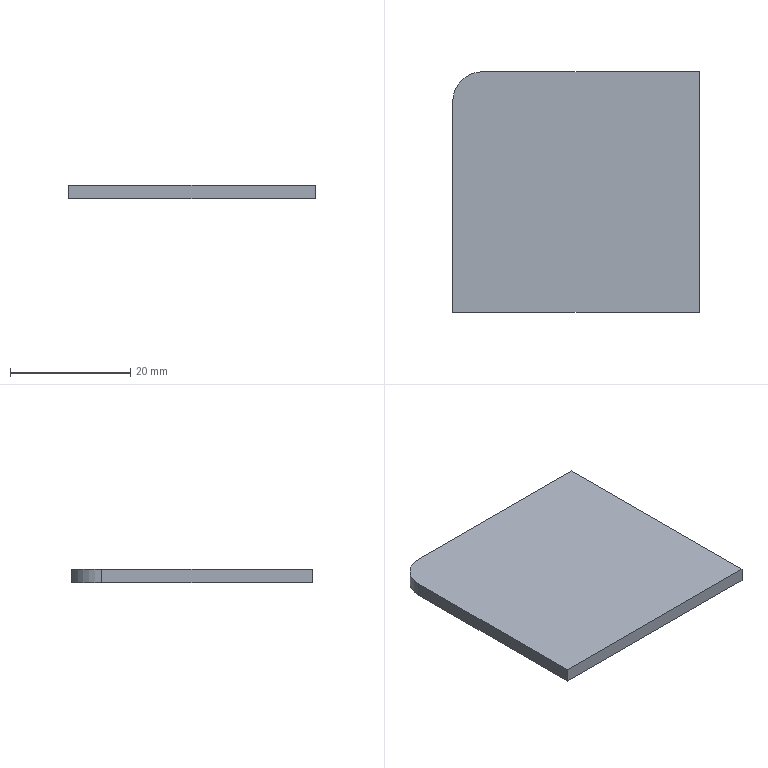Part | SolidWorks | features FlatPattern 1, SMBaseFlange 1, SheetMetal 1 | 1 solid | 7 faces | box 41 x 40 x 2.3 mm | volume 3760 mm3 | plane 6 | cylinder 1 | commonest cylinder face diameters 10 x1
STEP:
#1=CARTESIAN_POINT('',(41.,-40.,0.));
#2=VERTEX_POINT('',#1);
#3=CARTESIAN_POINT('',(41.,0.,0.));
#4=VERTEX_POINT('',#3);
#5=CARTESIAN_POINT('',(41.,0.,0.));
#6=DIRECTION('',(0.,1.,0.));
#7=VECTOR('',#6,1000.);
#8=LINE('',#5,#7);
#9=EDGE_CURVE('',#2,#4,#8,.T.);
#10=ORIENTED_EDGE('',*,*,#9,.F.);
#11=CARTESIAN_POINT('',(41.,-40.,-2.3));
#12=VERTEX_POINT('',#11);
#13=CARTESIAN_POINT('',(41.,-40.,-2.3));
#14=DIRECTION('',(0.,0.,1.));
#15=VECTOR('',#14,1000.);
#16=LINE('',#13,#15);
#17=EDGE_CURVE('',#12,#2,#16,.T.);
#18=ORIENTED_EDGE('',*,*,#17,.F.);
#19=CARTESIAN_POINT('',(41.,0.,-2.3));
#20=VERTEX_POINT('',#19);
#21=CARTESIAN_POINT('',(41.,0.,-2.3));
#22=DIRECTION('',(0.,1.,0.));
#23=VECTOR('',#22,1000.);
#24=LINE('',#21,#23);
#25=EDGE_CURVE('',#12,#20,#24,.T.);
#26=ORIENTED_EDGE('',*,*,#25,.T.);
#27=CARTESIAN_POINT('',(41.,0.,-2.3));
#28=DIRECTION('',(0.,0.,1.));
#29=VECTOR('',#28,1000.);
#30=LINE('',#27,#29);
#31=EDGE_CURVE('',#20,#4,#30,.T.);
#32=ORIENTED_EDGE('',*,*,#31,.T.);
#33=EDGE_LOOP('',(#10,#18,#26,#32));
#34=FACE_OUTER_BOUND('',#33,.T.);
#35=CARTESIAN_POINT('',(41.,0.,-2.3));
#36=DIRECTION('',(1.,0.,0.));
#37=DIRECTION('',(0.,1.,0.));
#38=AXIS2_PLACEMENT_3D('',#35,#36,#37);
#39=PLANE('',#38);
#40=ADVANCED_FACE('',(#34),#39,.T.);
#41=CARTESIAN_POINT('',(0.,-40.,0.));
#42=VERTEX_POINT('',#41);
#43=CARTESIAN_POINT('',(0.,-40.,0.));
#44=DIRECTION('',(1.,0.,0.));
#45=VECTOR('',#44,1000.);
#46=LINE('',#43,#45);
#47=EDGE_CURVE('',#42,#2,#46,.T.);
#48=ORIENTED_EDGE('',*,*,#47,.F.);
#49=CARTESIAN_POINT('',(0.,-40.,-2.3));
#50=VERTEX_POINT('',#49);
#51=CARTESIAN_POINT('',(0.,-40.,-2.3));
#52=DIRECTION('',(0.,0.,1.));
#53=VECTOR('',#52,1000.);
#54=LINE('',#51,#53);
#55=EDGE_CURVE('',#50,#42,#54,.T.);
#56=ORIENTED_EDGE('',*,*,#55,.F.);
#57=CARTESIAN_POINT('',(0.,-40.,-2.3));
#58=DIRECTION('',(1.,0.,0.));
#59=VECTOR('',#58,1000.);
#60=LINE('',#57,#59);
#61=EDGE_CURVE('',#50,#12,#60,.T.);
#62=ORIENTED_EDGE('',*,*,#61,.T.);
#63=ORIENTED_EDGE('',*,*,#17,.T.);
#64=EDGE_LOOP('',(#48,#56,#62,#63));
#65=FACE_OUTER_BOUND('',#64,.T.);
#66=CARTESIAN_POINT('',(0.,-40.,-2.3));
#67=DIRECTION('',(0.,-1.,0.));
#68=DIRECTION('',(0.,0.,-1.));
#69=AXIS2_PLACEMENT_3D('',#66,#67,#68);
#70=PLANE('',#69);
#71=ADVANCED_FACE('',(#65),#70,.T.);
#72=CARTESIAN_POINT('',(0.,-5.,0.));
#73=VERTEX_POINT('',#72);
#74=CARTESIAN_POINT('',(0.,-5.,0.));
#75=DIRECTION('',(0.,-1.,0.));
#76=VECTOR('',#75,1000.);
#77=LINE('',#74,#76);
#78=EDGE_CURVE('',#73,#42,#77,.T.);
#79=ORIENTED_EDGE('',*,*,#78,.F.);
#80=CARTESIAN_POINT('',(0.,-5.,-2.3));
#81=VERTEX_POINT('',#80);
#82=CARTESIAN_POINT('',(0.,-5.,-2.3));
#83=DIRECTION('',(0.,0.,1.));
#84=VECTOR('',#83,1000.);
#85=LINE('',#82,#84);
#86=EDGE_CURVE('',#81,#73,#85,.T.);
#87=ORIENTED_EDGE('',*,*,#86,.F.);
#88=CARTESIAN_POINT('',(0.,-5.,-2.3));
#89=DIRECTION('',(0.,-1.,0.));
#90=VECTOR('',#89,1000.);
#91=LINE('',#88,#90);
#92=EDGE_CURVE('',#81,#50,#91,.T.);
#93=ORIENTED_EDGE('',*,*,#92,.T.);
#94=ORIENTED_EDGE('',*,*,#55,.T.);
#95=EDGE_LOOP('',(#79,#87,#93,#94));
#96=FACE_OUTER_BOUND('',#95,.T.);
#97=CARTESIAN_POINT('',(0.,-5.,-2.3));
#98=DIRECTION('',(-1.,0.,0.));
#99=DIRECTION('',(0.,-1.,0.));
#100=AXIS2_PLACEMENT_3D('',#97,#98,#99);
#101=PLANE('',#100);
#102=ADVANCED_FACE('',(#96),#101,.T.);
#103=CARTESIAN_POINT('',(5.,0.,0.));
#104=VERTEX_POINT('',#103);
#105=CARTESIAN_POINT('',(5.,-5.,0.));
#106=DIRECTION('',(0.,0.,1.));
#107=DIRECTION('',(1.,0.,0.));
#108=AXIS2_PLACEMENT_3D('',#105,#106,#107);
#109=CIRCLE('',#108,5.);
#110=EDGE_CURVE('',#104,#73,#109,.T.);
#111=ORIENTED_EDGE('',*,*,#110,.F.);
#112=CARTESIAN_POINT('',(5.,0.,-2.3));
#113=VERTEX_POINT('',#112);
#114=CARTESIAN_POINT('',(5.,0.,-2.3));
#115=DIRECTION('',(0.,0.,1.));
#116=VECTOR('',#115,1000.);
#117=LINE('',#114,#116);
#118=EDGE_CURVE('',#113,#104,#117,.T.);
#119=ORIENTED_EDGE('',*,*,#118,.F.);
#120=CARTESIAN_POINT('',(5.,-5.,-2.3));
#121=DIRECTION('',(0.,0.,1.));
#122=DIRECTION('',(1.,0.,0.));
#123=AXIS2_PLACEMENT_3D('',#120,#121,#122);
#124=CIRCLE('',#123,5.);
#125=EDGE_CURVE('',#113,#81,#124,.T.);
#126=ORIENTED_EDGE('',*,*,#125,.T.);
#127=ORIENTED_EDGE('',*,*,#86,.T.);
#128=EDGE_LOOP('',(#111,#119,#126,#127));
#129=FACE_OUTER_BOUND('',#128,.T.);
#130=CARTESIAN_POINT('',(5.,-5.,-2.3));
#131=DIRECTION('',(0.,0.,1.));
#132=DIRECTION('',(1.,0.,0.));
#133=AXIS2_PLACEMENT_3D('',#130,#131,#132);
#134=CYLINDRICAL_SURFACE('',#133,5.);
#135=ADVANCED_FACE('',(#129),#134,.T.);
#136=CARTESIAN_POINT('',(5.,0.,0.));
#137=DIRECTION('',(-1.,0.,0.));
#138=VECTOR('',#137,1000.);
#139=LINE('',#136,#138);
#140=EDGE_CURVE('',#4,#104,#139,.T.);
#141=ORIENTED_EDGE('',*,*,#140,.F.);
#142=ORIENTED_EDGE('',*,*,#31,.F.);
#143=CARTESIAN_POINT('',(5.,0.,-2.3));
#144=DIRECTION('',(-1.,0.,0.));
#145=VECTOR('',#144,1000.);
#146=LINE('',#143,#145);
#147=EDGE_CURVE('',#20,#113,#146,.T.);
#148=ORIENTED_EDGE('',*,*,#147,.T.);
#149=ORIENTED_EDGE('',*,*,#118,.T.);
#150=EDGE_LOOP('',(#141,#142,#148,#149));
#151=FACE_OUTER_BOUND('',#150,.T.);
#152=CARTESIAN_POINT('',(5.,0.,-2.3));
#153=DIRECTION('',(0.,1.,0.));
#154=DIRECTION('',(0.,0.,1.));
#155=AXIS2_PLACEMENT_3D('',#152,#153,#154);
#156=PLANE('',#155);
#157=ADVANCED_FACE('',(#151),#156,.T.);
#158=ORIENTED_EDGE('',*,*,#25,.F.);
#159=ORIENTED_EDGE('',*,*,#61,.F.);
#160=ORIENTED_EDGE('',*,*,#92,.F.);
#161=ORIENTED_EDGE('',*,*,#125,.F.);
#162=ORIENTED_EDGE('',*,*,#147,.F.);
#163=EDGE_LOOP('',(#158,#159,#160,#161,#162));
#164=FACE_OUTER_BOUND('',#163,.T.);
#165=CARTESIAN_POINT('',(5.,-5.,-2.3));
#166=DIRECTION('',(0.,0.,1.));
#167=DIRECTION('',(1.,0.,0.));
#168=AXIS2_PLACEMENT_3D('',#165,#166,#167);
#169=PLANE('',#168);
#170=ADVANCED_FACE('',(#164),#169,.F.);
#171=ORIENTED_EDGE('',*,*,#9,.T.);
#172=ORIENTED_EDGE('',*,*,#140,.T.);
#173=ORIENTED_EDGE('',*,*,#110,.T.);
#174=ORIENTED_EDGE('',*,*,#78,.T.);
#175=ORIENTED_EDGE('',*,*,#47,.T.);
#176=EDGE_LOOP('',(#171,#172,#173,#174,#175));
#177=FACE_OUTER_BOUND('',#176,.T.);
#178=CARTESIAN_POINT('',(5.,-5.,0.));
#179=DIRECTION('',(0.,0.,1.));
#180=DIRECTION('',(1.,0.,0.));
#181=AXIS2_PLACEMENT_3D('',#178,#179,#180);
#182=PLANE('',#181);
#183=ADVANCED_FACE('',(#177),#182,.T.);
#184=CLOSED_SHELL('',(#40,#71,#102,#135,#157,#170,#183));
#185=MANIFOLD_SOLID_BREP('',#184);
#186=CARTESIAN_POINT('',(0.,0.,0.));
#187=DIRECTION('',(0.,0.,1.));
#188=DIRECTION('',(1.,0.,0.));
#189=AXIS2_PLACEMENT_3D('',#186,#187,#188);
#190=(LENGTH_UNIT()NAMED_UNIT(*)SI_UNIT(.MILLI.,.METRE.));
#191=UNCERTAINTY_MEASURE_WITH_UNIT(LENGTH_MEASURE(0.00001),#190,'','');
#192=(NAMED_UNIT(*)PLANE_ANGLE_UNIT()SI_UNIT($,.RADIAN.));
#193=(NAMED_UNIT(*)SI_UNIT($,.STERADIAN.)SOLID_ANGLE_UNIT());
#194=(GEOMETRIC_REPRESENTATION_CONTEXT(3)GLOBAL_UNCERTAINTY_ASSIGNED_CONTEXT((#191))GLOBAL_UNIT_ASSIGNED_CONTEXT((#190,#192,#193))REPRESENTATION_CONTEXT('',''));
#195=ADVANCED_BREP_SHAPE_REPRESENTATION('',(#185,#189),#194);